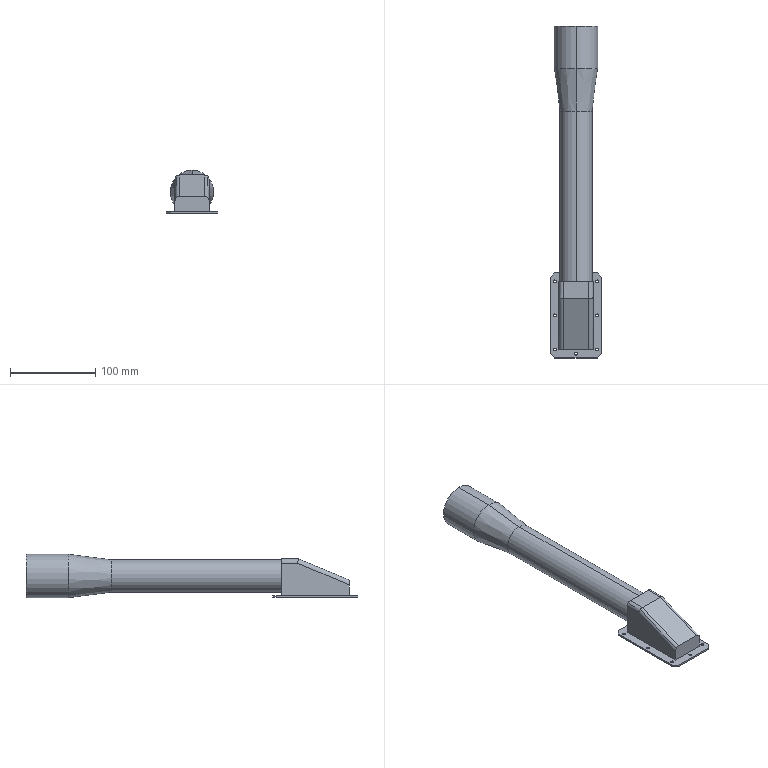Part | SolidWorks | features ICE 4, Chamfer 1, Cut 1, Extrusion 1, Fillet 1, MirrorPattern 1, Revolution 1, Shell 1 | 1 solid | 54 faces | box 60 x 390 x 51 mm | volume 98660 mm3 | cylinder 26 | plane 24 | cone 4 | commonest cylinder face diameters 3.5 x14 10 x4 34 x2 38 x2 47 x2 51 x2